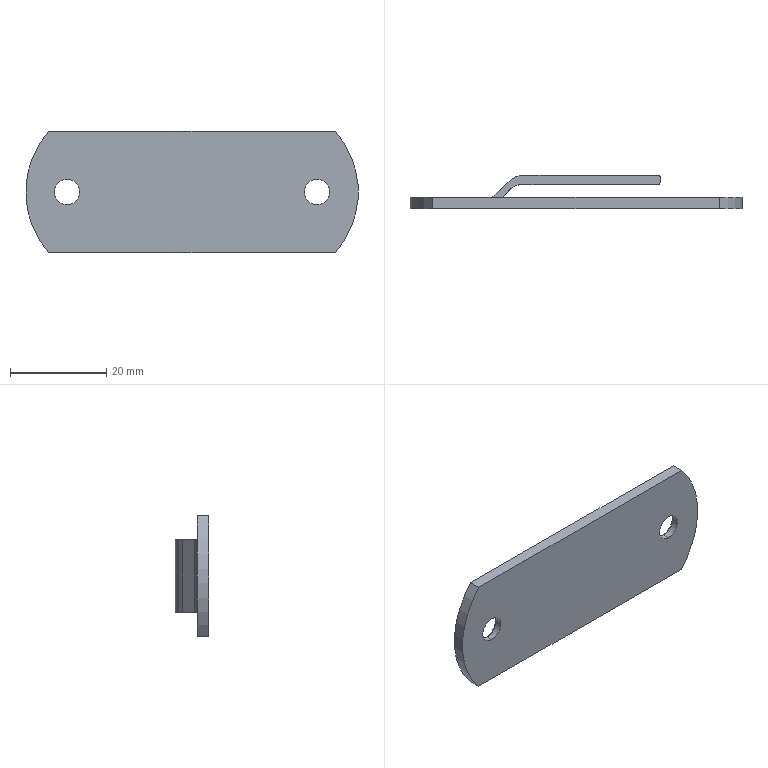Part | SolidWorks | features BaseBody 1 | 1 solid | 32 faces | box 69.2 x 7 x 25.2 mm | volume 3971 mm3 | plane 16 | cylinder 12 | cone 4 | commonest cylinder face diameters 5.3 x4 1 x2 6 x2 10 x2 37.875 x2
STEP:
#1=CARTESIAN_POINT('',(26.,-3.6,2.65));
#2=VERTEX_POINT('',#1);
#3=CARTESIAN_POINT('',(26.,-3.6,-2.65));
#4=VERTEX_POINT('',#3);
#5=CARTESIAN_POINT('',(26.,-3.6,0.));
#6=DIRECTION('',(0.,-1.,0.));
#7=DIRECTION('',(0.,0.,1.));
#8=AXIS2_PLACEMENT_3D('',#5,#6,#7);
#9=CIRCLE('',#8,2.65);
#10=EDGE_CURVE('',#2,#4,#9,.T.);
#11=ORIENTED_EDGE('',*,*,#10,.T.);
#12=CARTESIAN_POINT('',(26.,-2.2,-2.65));
#13=VERTEX_POINT('',#12);
#14=CARTESIAN_POINT('',(26.,-3.6,-2.65));
#15=DIRECTION('',(0.,1.,0.));
#16=VECTOR('',#15,1000.);
#17=LINE('',#14,#16);
#18=EDGE_CURVE('',#4,#13,#17,.T.);
#19=ORIENTED_EDGE('',*,*,#18,.T.);
#20=CARTESIAN_POINT('',(26.,-2.2,2.65));
#21=VERTEX_POINT('',#20);
#22=CARTESIAN_POINT('',(26.,-2.2,0.));
#23=DIRECTION('',(0.,-1.,0.));
#24=DIRECTION('',(0.,0.,1.));
#25=AXIS2_PLACEMENT_3D('',#22,#23,#24);
#26=CIRCLE('',#25,2.65);
#27=EDGE_CURVE('',#21,#13,#26,.T.);
#28=ORIENTED_EDGE('',*,*,#27,.F.);
#29=CARTESIAN_POINT('',(26.,-3.6,2.65));
#30=DIRECTION('',(0.,1.,0.));
#31=VECTOR('',#30,1000.);
#32=LINE('',#29,#31);
#33=EDGE_CURVE('',#2,#21,#32,.T.);
#34=ORIENTED_EDGE('',*,*,#33,.F.);
#35=EDGE_LOOP('',(#11,#19,#28,#34));
#36=FACE_OUTER_BOUND('',#35,.T.);
#37=CARTESIAN_POINT('',(26.,-3.6,0.));
#38=DIRECTION('',(0.,1.,0.));
#39=DIRECTION('',(0.,0.,1.));
#40=AXIS2_PLACEMENT_3D('',#37,#38,#39);
#41=CYLINDRICAL_SURFACE('',#40,2.65);
#42=ADVANCED_FACE('',(#36),#41,.F.);
#43=CARTESIAN_POINT('',(-26.,-3.6,2.65));
#44=VERTEX_POINT('',#43);
#45=CARTESIAN_POINT('',(-26.,-3.6,-2.65));
#46=VERTEX_POINT('',#45);
#47=CARTESIAN_POINT('',(-26.,-3.6,0.));
#48=DIRECTION('',(0.,-1.,0.));
#49=DIRECTION('',(0.,0.,1.));
#50=AXIS2_PLACEMENT_3D('',#47,#48,#49);
#51=CIRCLE('',#50,2.65);
#52=EDGE_CURVE('',#44,#46,#51,.T.);
#53=ORIENTED_EDGE('',*,*,#52,.T.);
#54=CARTESIAN_POINT('',(-26.,-2.2,-2.65));
#55=VERTEX_POINT('',#54);
#56=CARTESIAN_POINT('',(-26.,-3.6,-2.65));
#57=DIRECTION('',(0.,1.,0.));
#58=VECTOR('',#57,1000.);
#59=LINE('',#56,#58);
#60=EDGE_CURVE('',#46,#55,#59,.T.);
#61=ORIENTED_EDGE('',*,*,#60,.T.);
#62=CARTESIAN_POINT('',(-26.,-2.2,2.65));
#63=VERTEX_POINT('',#62);
#64=CARTESIAN_POINT('',(-26.,-2.2,0.));
#65=DIRECTION('',(0.,-1.,0.));
#66=DIRECTION('',(0.,0.,1.));
#67=AXIS2_PLACEMENT_3D('',#64,#65,#66);
#68=CIRCLE('',#67,2.65);
#69=EDGE_CURVE('',#63,#55,#68,.T.);
#70=ORIENTED_EDGE('',*,*,#69,.F.);
#71=CARTESIAN_POINT('',(-26.,-3.6,2.65));
#72=DIRECTION('',(0.,1.,0.));
#73=VECTOR('',#72,1000.);
#74=LINE('',#71,#73);
#75=EDGE_CURVE('',#44,#63,#74,.T.);
#76=ORIENTED_EDGE('',*,*,#75,.F.);
#77=EDGE_LOOP('',(#53,#61,#70,#76));
#78=FACE_OUTER_BOUND('',#77,.T.);
#79=CARTESIAN_POINT('',(-26.,-3.6,0.));
#80=DIRECTION('',(0.,1.,0.));
#81=DIRECTION('',(0.,0.,1.));
#82=AXIS2_PLACEMENT_3D('',#79,#80,#81);
#83=CYLINDRICAL_SURFACE('',#82,2.65);
#84=ADVANCED_FACE('',(#78),#83,.F.);
#85=ORIENTED_EDGE('',*,*,#27,.T.);
#86=CARTESIAN_POINT('',(26.,-1.2,-3.8));
#87=VERTEX_POINT('',#86);
#88=CARTESIAN_POINT('',(26.,-1.2,-3.8));
#89=DIRECTION('',(0.,0.6562,-0.7546));
#90=VECTOR('',#89,1000.);
#91=LINE('',#88,#90);
#92=EDGE_CURVE('',#13,#87,#91,.T.);
#93=ORIENTED_EDGE('',*,*,#92,.T.);
#94=CARTESIAN_POINT('',(26.,-1.2,3.8));
#95=VERTEX_POINT('',#94);
#96=CARTESIAN_POINT('',(26.,-1.2,0.));
#97=DIRECTION('',(0.,-1.,0.));
#98=DIRECTION('',(0.,0.,1.));
#99=AXIS2_PLACEMENT_3D('',#96,#97,#98);
#100=CIRCLE('',#99,3.8);
#101=EDGE_CURVE('',#95,#87,#100,.T.);
#102=ORIENTED_EDGE('',*,*,#101,.F.);
#103=CARTESIAN_POINT('',(26.,-1.2,3.8));
#104=DIRECTION('',(0.,0.6562,0.7546));
#105=VECTOR('',#104,1000.);
#106=LINE('',#103,#105);
#107=EDGE_CURVE('',#21,#95,#106,.T.);
#108=ORIENTED_EDGE('',*,*,#107,.F.);
#109=EDGE_LOOP('',(#85,#93,#102,#108));
#110=FACE_OUTER_BOUND('',#109,.T.);
#111=CARTESIAN_POINT('',(26.,-1.2,0.));
#112=DIRECTION('',(0.,1.,0.));
#113=DIRECTION('',(0.,0.,1.));
#114=AXIS2_PLACEMENT_3D('',#111,#112,#113);
#115=CONICAL_SURFACE('',#114,3.8,0.8551);
#116=ADVANCED_FACE('',(#110),#115,.F.);
#117=ORIENTED_EDGE('',*,*,#69,.T.);
#118=CARTESIAN_POINT('',(-26.,-1.2,-3.8));
#119=VERTEX_POINT('',#118);
#120=CARTESIAN_POINT('',(-26.,-1.2,-3.8));
#121=DIRECTION('',(0.,0.6562,-0.7546));
#122=VECTOR('',#121,1000.);
#123=LINE('',#120,#122);
#124=EDGE_CURVE('',#55,#119,#123,.T.);
#125=ORIENTED_EDGE('',*,*,#124,.T.);
#126=CARTESIAN_POINT('',(-26.,-1.2,3.8));
#127=VERTEX_POINT('',#126);
#128=CARTESIAN_POINT('',(-26.,-1.2,0.));
#129=DIRECTION('',(0.,-1.,0.));
#130=DIRECTION('',(0.,0.,1.));
#131=AXIS2_PLACEMENT_3D('',#128,#129,#130);
#132=CIRCLE('',#131,3.8);
#133=EDGE_CURVE('',#127,#119,#132,.T.);
#134=ORIENTED_EDGE('',*,*,#133,.F.);
#135=CARTESIAN_POINT('',(-26.,-1.2,3.8));
#136=DIRECTION('',(0.,0.6562,0.7546));
#137=VECTOR('',#136,1000.);
#138=LINE('',#135,#137);
#139=EDGE_CURVE('',#63,#127,#138,.T.);
#140=ORIENTED_EDGE('',*,*,#139,.F.);
#141=EDGE_LOOP('',(#117,#125,#134,#140));
#142=FACE_OUTER_BOUND('',#141,.T.);
#143=CARTESIAN_POINT('',(-26.,-1.2,0.));
#144=DIRECTION('',(0.,1.,0.));
#145=DIRECTION('',(0.,0.,1.));
#146=AXIS2_PLACEMENT_3D('',#143,#144,#145);
#147=CONICAL_SURFACE('',#146,3.8,0.8551);
#148=ADVANCED_FACE('',(#142),#147,.F.);
#149=CARTESIAN_POINT('',(29.8,-3.6,12.6));
#150=VERTEX_POINT('',#149);
#151=CARTESIAN_POINT('',(29.8,-3.6,-12.6));
#152=VERTEX_POINT('',#151);
#153=CARTESIAN_POINT('',(15.662,-3.6,0.));
#154=DIRECTION('',(0.,1.,0.));
#155=DIRECTION('',(0.,0.,-1.));
#156=AXIS2_PLACEMENT_3D('',#153,#154,#155);
#157=CIRCLE('',#156,18.938);
#158=EDGE_CURVE('',#150,#152,#157,.T.);
#159=ORIENTED_EDGE('',*,*,#158,.F.);
#160=CARTESIAN_POINT('',(-29.8,-3.6,12.6));
#161=VERTEX_POINT('',#160);
#162=CARTESIAN_POINT('',(-15.662,-3.6,12.6));
#163=DIRECTION('',(1.,0.,0.));
#164=VECTOR('',#163,1000.);
#165=LINE('',#162,#164);
#166=EDGE_CURVE('',#161,#150,#165,.T.);
#167=ORIENTED_EDGE('',*,*,#166,.F.);
#168=CARTESIAN_POINT('',(-29.8,-3.6,-12.6));
#169=VERTEX_POINT('',#168);
#170=CARTESIAN_POINT('',(-15.662,-3.6,0.));
#171=DIRECTION('',(0.,1.,0.));
#172=DIRECTION('',(0.,0.,-1.));
#173=AXIS2_PLACEMENT_3D('',#170,#171,#172);
#174=CIRCLE('',#173,18.938);
#175=EDGE_CURVE('',#169,#161,#174,.T.);
#176=ORIENTED_EDGE('',*,*,#175,.F.);
#177=CARTESIAN_POINT('',(-15.662,-3.6,-12.6));
#178=DIRECTION('',(-1.,0.,0.));
#179=VECTOR('',#178,1000.);
#180=LINE('',#177,#179);
#181=EDGE_CURVE('',#152,#169,#180,.T.);
#182=ORIENTED_EDGE('',*,*,#181,.F.);
#183=EDGE_LOOP('',(#159,#167,#176,#182));
#184=FACE_OUTER_BOUND('',#183,.T.);
#185=ORIENTED_EDGE('',*,*,#10,.F.);
#186=CARTESIAN_POINT('',(26.,-3.6,0.));
#187=DIRECTION('',(0.,-1.,0.));
#188=DIRECTION('',(0.,0.,1.));
#189=AXIS2_PLACEMENT_3D('',#186,#187,#188);
#190=CIRCLE('',#189,2.65);
#191=EDGE_CURVE('',#4,#2,#190,.T.);
#192=ORIENTED_EDGE('',*,*,#191,.F.);
#193=EDGE_LOOP('',(#185,#192));
#194=FACE_BOUND('',#193,.T.);
#195=ORIENTED_EDGE('',*,*,#52,.F.);
#196=CARTESIAN_POINT('',(-26.,-3.6,0.));
#197=DIRECTION('',(0.,-1.,0.));
#198=DIRECTION('',(0.,0.,1.));
#199=AXIS2_PLACEMENT_3D('',#196,#197,#198);
#200=CIRCLE('',#199,2.65);
#201=EDGE_CURVE('',#46,#44,#200,.T.);
#202=ORIENTED_EDGE('',*,*,#201,.F.);
#203=EDGE_LOOP('',(#195,#202));
#204=FACE_BOUND('',#203,.T.);
#205=CARTESIAN_POINT('',(-15.662,-3.6,0.));
#206=DIRECTION('',(0.,1.,0.));
#207=DIRECTION('',(0.,0.,1.));
#208=AXIS2_PLACEMENT_3D('',#205,#206,#207);
#209=PLANE('',#208);
#210=ADVANCED_FACE('',(#184,#194,#204),#209,.F.);
#211=ORIENTED_EDGE('',*,*,#181,.T.);
#212=CARTESIAN_POINT('',(-29.8,-1.2,-12.6));
#213=VERTEX_POINT('',#212);
#214=CARTESIAN_POINT('',(-29.8,-3.6,-12.6));
#215=DIRECTION('',(0.,1.,0.));
#216=VECTOR('',#215,1000.);
#217=LINE('',#214,#216);
#218=EDGE_CURVE('',#169,#213,#217,.T.);
#219=ORIENTED_EDGE('',*,*,#218,.T.);
#220=CARTESIAN_POINT('',(29.8,-1.2,-12.6));
#221=VERTEX_POINT('',#220);
#222=CARTESIAN_POINT('',(29.8,-1.2,-12.6));
#223=DIRECTION('',(1.,0.,0.));
#224=VECTOR('',#223,1000.);
#225=LINE('',#222,#224);
#226=EDGE_CURVE('',#213,#221,#225,.T.);
#227=ORIENTED_EDGE('',*,*,#226,.T.);
#228=CARTESIAN_POINT('',(29.8,-3.6,-12.6));
#229=DIRECTION('',(0.,-1.,0.));
#230=VECTOR('',#229,1000.);
#231=LINE('',#228,#230);
#232=EDGE_CURVE('',#221,#152,#231,.T.);
#233=ORIENTED_EDGE('',*,*,#232,.T.);
#234=EDGE_LOOP('',(#211,#219,#227,#233));
#235=FACE_OUTER_BOUND('',#234,.T.);
#236=CARTESIAN_POINT('',(29.8,-3.6,-12.6));
#237=DIRECTION('',(0.,0.,-1.));
#238=DIRECTION('',(-1.,0.,0.));
#239=AXIS2_PLACEMENT_3D('',#236,#237,#238);
#240=PLANE('',#239);
#241=ADVANCED_FACE('',(#235),#240,.T.);
#242=ORIENTED_EDGE('',*,*,#158,.T.);
#243=ORIENTED_EDGE('',*,*,#232,.F.);
#244=CARTESIAN_POINT('',(29.8,-1.2,12.6));
#245=VERTEX_POINT('',#244);
#246=CARTESIAN_POINT('',(15.662,-1.2,0.));
#247=DIRECTION('',(0.,-1.,0.));
#248=DIRECTION('',(0.,0.,-1.));
#249=AXIS2_PLACEMENT_3D('',#246,#247,#248);
#250=CIRCLE('',#249,18.938);
#251=EDGE_CURVE('',#221,#245,#250,.T.);
#252=ORIENTED_EDGE('',*,*,#251,.T.);
#253=CARTESIAN_POINT('',(29.8,-3.6,12.6));
#254=DIRECTION('',(0.,-1.,0.));
#255=VECTOR('',#254,1000.);
#256=LINE('',#253,#255);
#257=EDGE_CURVE('',#245,#150,#256,.T.);
#258=ORIENTED_EDGE('',*,*,#257,.T.);
#259=EDGE_LOOP('',(#242,#243,#252,#258));
#260=FACE_OUTER_BOUND('',#259,.T.);
#261=CARTESIAN_POINT('',(15.662,-3.6,0.));
#262=DIRECTION('',(0.,-1.,0.));
#263=DIRECTION('',(0.,0.,-1.));
#264=AXIS2_PLACEMENT_3D('',#261,#262,#263);
#265=CYLINDRICAL_SURFACE('',#264,18.938);
#266=ADVANCED_FACE('',(#260),#265,.T.);
#267=ORIENTED_EDGE('',*,*,#166,.T.);
#268=ORIENTED_EDGE('',*,*,#257,.F.);
#269=CARTESIAN_POINT('',(-29.8,-1.2,12.6));
#270=VERTEX_POINT('',#269);
#271=CARTESIAN_POINT('',(-29.8,-1.2,12.6));
#272=DIRECTION('',(-1.,0.,0.));
#273=VECTOR('',#272,1000.);
#274=LINE('',#271,#273);
#275=EDGE_CURVE('',#245,#270,#274,.T.);
#276=ORIENTED_EDGE('',*,*,#275,.T.);
#277=CARTESIAN_POINT('',(-29.8,-3.6,12.6));
#278=DIRECTION('',(0.,-1.,0.));
#279=VECTOR('',#278,1000.);
#280=LINE('',#277,#279);
#281=EDGE_CURVE('',#270,#161,#280,.T.);
#282=ORIENTED_EDGE('',*,*,#281,.T.);
#283=EDGE_LOOP('',(#267,#268,#276,#282));
#284=FACE_OUTER_BOUND('',#283,.T.);
#285=CARTESIAN_POINT('',(-29.8,-3.6,12.6));
#286=DIRECTION('',(0.,0.,1.));
#287=DIRECTION('',(1.,0.,0.));
#288=AXIS2_PLACEMENT_3D('',#285,#286,#287);
#289=PLANE('',#288);
#290=ADVANCED_FACE('',(#284),#289,.T.);
#291=ORIENTED_EDGE('',*,*,#175,.T.);
#292=ORIENTED_EDGE('',*,*,#281,.F.);
#293=CARTESIAN_POINT('',(-15.662,-1.2,0.));
#294=DIRECTION('',(0.,-1.,0.));
#295=DIRECTION('',(0.,0.,-1.));
#296=AXIS2_PLACEMENT_3D('',#293,#294,#295);
#297=CIRCLE('',#296,18.938);
#298=EDGE_CURVE('',#270,#213,#297,.T.);
#299=ORIENTED_EDGE('',*,*,#298,.T.);
#300=ORIENTED_EDGE('',*,*,#218,.F.);
#301=EDGE_LOOP('',(#291,#292,#299,#300));
#302=FACE_OUTER_BOUND('',#301,.T.);
#303=CARTESIAN_POINT('',(-15.662,-3.6,0.));
#304=DIRECTION('',(0.,-1.,0.));
#305=DIRECTION('',(0.,0.,-1.));
#306=AXIS2_PLACEMENT_3D('',#303,#304,#305);
#307=CYLINDRICAL_SURFACE('',#306,18.938);
#308=ADVANCED_FACE('',(#302),#307,.T.);
#309=ORIENTED_EDGE('',*,*,#18,.F.);
#310=ORIENTED_EDGE('',*,*,#191,.T.);
#311=ORIENTED_EDGE('',*,*,#33,.T.);
#312=CARTESIAN_POINT('',(26.,-2.2,0.));
#313=DIRECTION('',(0.,-1.,0.));
#314=DIRECTION('',(0.,0.,1.));
#315=AXIS2_PLACEMENT_3D('',#312,#313,#314);
#316=CIRCLE('',#315,2.65);
#317=EDGE_CURVE('',#13,#21,#316,.T.);
#318=ORIENTED_EDGE('',*,*,#317,.F.);
#319=EDGE_LOOP('',(#309,#310,#311,#318));
#320=FACE_OUTER_BOUND('',#319,.T.);
#321=CARTESIAN_POINT('',(26.,-3.6,0.));
#322=DIRECTION('',(0.,1.,0.));
#323=DIRECTION('',(0.,0.,1.));
#324=AXIS2_PLACEMENT_3D('',#321,#322,#323);
#325=CYLINDRICAL_SURFACE('',#324,2.65);
#326=ADVANCED_FACE('',(#320),#325,.F.);
#327=ORIENTED_EDGE('',*,*,#60,.F.);
#328=ORIENTED_EDGE('',*,*,#201,.T.);
#329=ORIENTED_EDGE('',*,*,#75,.T.);
#330=CARTESIAN_POINT('',(-26.,-2.2,0.));
#331=DIRECTION('',(0.,-1.,0.));
#332=DIRECTION('',(0.,0.,1.));
#333=AXIS2_PLACEMENT_3D('',#330,#331,#332);
#334=CIRCLE('',#333,2.65);
#335=EDGE_CURVE('',#55,#63,#334,.T.);
#336=ORIENTED_EDGE('',*,*,#335,.F.);
#337=EDGE_LOOP('',(#327,#328,#329,#336));
#338=FACE_OUTER_BOUND('',#337,.T.);
#339=CARTESIAN_POINT('',(-26.,-3.6,0.));
#340=DIRECTION('',(0.,1.,0.));
#341=DIRECTION('',(0.,0.,1.));
#342=AXIS2_PLACEMENT_3D('',#339,#340,#341);
#343=CYLINDRICAL_SURFACE('',#342,2.65);
#344=ADVANCED_FACE('',(#338),#343,.F.);
#345=ORIENTED_EDGE('',*,*,#275,.F.);
#346=ORIENTED_EDGE('',*,*,#251,.F.);
#347=ORIENTED_EDGE('',*,*,#226,.F.);
#348=ORIENTED_EDGE('',*,*,#298,.F.);
#349=EDGE_LOOP('',(#345,#346,#347,#348));
#350=FACE_OUTER_BOUND('',#349,.T.);
#351=ORIENTED_EDGE('',*,*,#101,.T.);
#352=CARTESIAN_POINT('',(26.,-1.2,0.));
#353=DIRECTION('',(0.,-1.,0.));
#354=DIRECTION('',(0.,0.,1.));
#355=AXIS2_PLACEMENT_3D('',#352,#353,#354);
#356=CIRCLE('',#355,3.8);
#357=EDGE_CURVE('',#87,#95,#356,.T.);
#358=ORIENTED_EDGE('',*,*,#357,.T.);
#359=EDGE_LOOP('',(#351,#358));
#360=FACE_BOUND('',#359,.T.);
#361=ORIENTED_EDGE('',*,*,#133,.T.);
#362=CARTESIAN_POINT('',(-26.,-1.2,0.));
#363=DIRECTION('',(0.,-1.,0.));
#364=DIRECTION('',(0.,0.,1.));
#365=AXIS2_PLACEMENT_3D('',#362,#363,#364);
#366=CIRCLE('',#365,3.8);
#367=EDGE_CURVE('',#119,#127,#366,.T.);
#368=ORIENTED_EDGE('',*,*,#367,.T.);
#369=EDGE_LOOP('',(#361,#368));
#370=FACE_BOUND('',#369,.T.);
#371=CARTESIAN_POINT('',(17.5,-1.2,-7.5));
#372=VERTEX_POINT('',#371);
#373=CARTESIAN_POINT('',(17.5,-1.2,7.5));
#374=VERTEX_POINT('',#373);
#375=CARTESIAN_POINT('',(17.5,-1.2,0.));
#376=DIRECTION('',(0.,0.,1.));
#377=VECTOR('',#376,1000.);
#378=LINE('',#375,#377);
#379=EDGE_CURVE('',#372,#374,#378,.T.);
#380=ORIENTED_EDGE('',*,*,#379,.T.);
#381=CARTESIAN_POINT('',(-15.3,-1.2,7.5));
#382=VERTEX_POINT('',#381);
#383=CARTESIAN_POINT('',(-15.662,-1.2,7.5));
#384=DIRECTION('',(-1.,0.,0.));
#385=VECTOR('',#384,1000.);
#386=LINE('',#383,#385);
#387=EDGE_CURVE('',#374,#382,#386,.T.);
#388=ORIENTED_EDGE('',*,*,#387,.T.);
#389=CARTESIAN_POINT('',(-17.666,-1.2,7.5));
#390=VERTEX_POINT('',#389);
#391=CARTESIAN_POINT('',(-15.662,-1.2,7.5));
#392=DIRECTION('',(-1.,0.,0.));
#393=VECTOR('',#392,1000.);
#394=LINE('',#391,#393);
#395=EDGE_CURVE('',#382,#390,#394,.T.);
#396=ORIENTED_EDGE('',*,*,#395,.T.);
#397=CARTESIAN_POINT('',(-17.666,-1.2,-7.5));
#398=VERTEX_POINT('',#397);
#399=CARTESIAN_POINT('',(-17.666,-1.2,0.));
#400=DIRECTION('',(0.,0.,-1.));
#401=VECTOR('',#400,1000.);
#402=LINE('',#399,#401);
#403=EDGE_CURVE('',#390,#398,#402,.T.);
#404=ORIENTED_EDGE('',*,*,#403,.T.);
#405=CARTESIAN_POINT('',(-15.3,-1.2,-7.5));
#406=VERTEX_POINT('',#405);
#407=CARTESIAN_POINT('',(-15.662,-1.2,-7.5));
#408=DIRECTION('',(1.,0.,0.));
#409=VECTOR('',#408,1000.);
#410=LINE('',#407,#409);
#411=EDGE_CURVE('',#398,#406,#410,.T.);
#412=ORIENTED_EDGE('',*,*,#411,.T.);
#413=CARTESIAN_POINT('',(-15.662,-1.2,-7.5));
#414=DIRECTION('',(1.,0.,0.));
#415=VECTOR('',#414,1000.);
#416=LINE('',#413,#415);
#417=EDGE_CURVE('',#406,#372,#416,.T.);
#418=ORIENTED_EDGE('',*,*,#417,.T.);
#419=EDGE_LOOP('',(#380,#388,#396,#404,#412,#418));
#420=FACE_BOUND('',#419,.T.);
#421=CARTESIAN_POINT('',(-15.662,-1.2,0.));
#422=DIRECTION('',(0.,1.,0.));
#423=DIRECTION('',(0.,0.,1.));
#424=AXIS2_PLACEMENT_3D('',#421,#422,#423);
#425=PLANE('',#424);
#426=ADVANCED_FACE('',(#350,#360,#370,#420),#425,.T.);
#427=ORIENTED_EDGE('',*,*,#92,.F.);
#428=ORIENTED_EDGE('',*,*,#317,.T.);
#429=ORIENTED_EDGE('',*,*,#107,.T.);
#430=ORIENTED_EDGE('',*,*,#357,.F.);
#431=EDGE_LOOP('',(#427,#428,#429,#430));
#432=FACE_OUTER_BOUND('',#431,.T.);
#433=CARTESIAN_POINT('',(26.,-1.2,0.));
#434=DIRECTION('',(0.,1.,0.));
#435=DIRECTION('',(0.,0.,1.));
#436=AXIS2_PLACEMENT_3D('',#433,#434,#435);
#437=CONICAL_SURFACE('',#436,3.8,0.8551);
#438=ADVANCED_FACE('',(#432),#437,.F.);
#439=ORIENTED_EDGE('',*,*,#124,.F.);
#440=ORIENTED_EDGE('',*,*,#335,.T.);
#441=ORIENTED_EDGE('',*,*,#139,.T.);
#442=ORIENTED_EDGE('',*,*,#367,.F.);
#443=EDGE_LOOP('',(#439,#440,#441,#442));
#444=FACE_OUTER_BOUND('',#443,.T.);
#445=CARTESIAN_POINT('',(-26.,-1.2,0.));
#446=DIRECTION('',(0.,1.,0.));
#447=DIRECTION('',(0.,0.,1.));
#448=AXIS2_PLACEMENT_3D('',#445,#446,#447);
#449=CONICAL_SURFACE('',#448,3.8,0.8551);
#450=ADVANCED_FACE('',(#444),#449,.F.);
#451=CARTESIAN_POINT('',(-16.036,-1.936,7.5));
#452=VERTEX_POINT('',#451);
#453=CARTESIAN_POINT('',(-16.036,-1.936,7.5));
#454=DIRECTION('',(0.7071,0.7071,0.));
#455=VECTOR('',#454,1000.);
#456=LINE('',#453,#455);
#457=EDGE_CURVE('',#452,#382,#456,.T.);
#458=ORIENTED_EDGE('',*,*,#457,.T.);
#459=ORIENTED_EDGE('',*,*,#387,.F.);
#460=CARTESIAN_POINT('',(17.5,-3.,7.5));
#461=VERTEX_POINT('',#460);
#462=CARTESIAN_POINT('',(17.5,0.,7.5));
#463=DIRECTION('',(0.,1.,0.));
#464=VECTOR('',#463,1000.);
#465=LINE('',#462,#464);
#466=EDGE_CURVE('',#461,#374,#465,.T.);
#467=ORIENTED_EDGE('',*,*,#466,.F.);
#468=CARTESIAN_POINT('',(-17.5,-3.,7.5));
#469=VERTEX_POINT('',#468);
#470=CARTESIAN_POINT('',(0.,-3.,7.5));
#471=DIRECTION('',(1.,0.,0.));
#472=VECTOR('',#471,1000.);
#473=LINE('',#470,#472);
#474=EDGE_CURVE('',#469,#461,#473,.T.);
#475=ORIENTED_EDGE('',*,*,#474,.F.);
#476=CARTESIAN_POINT('',(-17.5,-2.951,7.5));
#477=VERTEX_POINT('',#476);
#478=CARTESIAN_POINT('',(-17.5,3.,7.5));
#479=DIRECTION('',(0.,-1.,0.));
#480=VECTOR('',#479,1000.);
#481=LINE('',#478,#480);
#482=EDGE_CURVE('',#477,#469,#481,.T.);
#483=ORIENTED_EDGE('',*,*,#482,.F.);
#484=CARTESIAN_POINT('',(-19.571,1.6,7.5));
#485=DIRECTION('',(0.,0.,-1.));
#486=DIRECTION('',(1.,0.,0.));
#487=AXIS2_PLACEMENT_3D('',#484,#485,#486);
#488=CIRCLE('',#487,5.);
#489=EDGE_CURVE('',#452,#477,#488,.T.);
#490=ORIENTED_EDGE('',*,*,#489,.F.);
#491=EDGE_LOOP('',(#458,#459,#467,#475,#483,#490));
#492=FACE_OUTER_BOUND('',#491,.T.);
#493=CARTESIAN_POINT('',(0.,0.,7.5));
#494=DIRECTION('',(0.,0.,1.));
#495=DIRECTION('',(1.,0.,0.));
#496=AXIS2_PLACEMENT_3D('',#493,#494,#495);
#497=PLANE('',#496);
#498=ADVANCED_FACE('',(#492),#497,.F.);
#499=ORIENTED_EDGE('',*,*,#466,.T.);
#500=ORIENTED_EDGE('',*,*,#379,.F.);
#501=CARTESIAN_POINT('',(17.5,-3.,-7.5));
#502=VERTEX_POINT('',#501);
#503=CARTESIAN_POINT('',(17.5,-3.,-7.5));
#504=DIRECTION('',(0.,-1.,0.));
#505=VECTOR('',#504,1000.);
#506=LINE('',#503,#505);
#507=EDGE_CURVE('',#372,#502,#506,.T.);
#508=ORIENTED_EDGE('',*,*,#507,.T.);
#509=CARTESIAN_POINT('',(17.5,-3.,7.5));
#510=DIRECTION('',(0.,0.,1.));
#511=VECTOR('',#510,1000.);
#512=LINE('',#509,#511);
#513=EDGE_CURVE('',#502,#461,#512,.T.);
#514=ORIENTED_EDGE('',*,*,#513,.T.);
#515=EDGE_LOOP('',(#499,#500,#508,#514));
#516=FACE_OUTER_BOUND('',#515,.T.);
#517=CARTESIAN_POINT('',(17.5,-3.,7.5));
#518=DIRECTION('',(-1.,0.,0.));
#519=DIRECTION('',(0.,0.,1.));
#520=AXIS2_PLACEMENT_3D('',#517,#518,#519);
#521=PLANE('',#520);
#522=ADVANCED_FACE('',(#516),#521,.T.);
#523=ORIENTED_EDGE('',*,*,#507,.F.);
#524=ORIENTED_EDGE('',*,*,#417,.F.);
#525=CARTESIAN_POINT('',(-16.036,-1.936,-7.5));
#526=VERTEX_POINT('',#525);
#527=CARTESIAN_POINT('',(-16.036,-1.936,-7.5));
#528=DIRECTION('',(-0.7071,-0.7071,0.));
#529=VECTOR('',#528,1000.);
#530=LINE('',#527,#529);
#531=EDGE_CURVE('',#406,#526,#530,.T.);
#532=ORIENTED_EDGE('',*,*,#531,.T.);
#533=CARTESIAN_POINT('',(-17.5,-2.951,-7.5));
#534=VERTEX_POINT('',#533);
#535=CARTESIAN_POINT('',(-19.571,1.6,-7.5));
#536=DIRECTION('',(0.,0.,-1.));
#537=DIRECTION('',(1.,0.,0.));
#538=AXIS2_PLACEMENT_3D('',#535,#536,#537);
#539=CIRCLE('',#538,5.);
#540=EDGE_CURVE('',#526,#534,#539,.T.);
#541=ORIENTED_EDGE('',*,*,#540,.T.);
#542=CARTESIAN_POINT('',(-17.5,-3.,-7.5));
#543=VERTEX_POINT('',#542);
#544=CARTESIAN_POINT('',(-17.5,3.,-7.5));
#545=DIRECTION('',(0.,1.,0.));
#546=VECTOR('',#545,1000.);
#547=LINE('',#544,#546);
#548=EDGE_CURVE('',#543,#534,#547,.T.);
#549=ORIENTED_EDGE('',*,*,#548,.F.);
#550=CARTESIAN_POINT('',(0.,-3.,-7.5));
#551=DIRECTION('',(1.,0.,0.));
#552=VECTOR('',#551,1000.);
#553=LINE('',#550,#552);
#554=EDGE_CURVE('',#543,#502,#553,.T.);
#555=ORIENTED_EDGE('',*,*,#554,.T.);
#556=EDGE_LOOP('',(#523,#524,#532,#541,#549,#555));
#557=FACE_OUTER_BOUND('',#556,.T.);
#558=CARTESIAN_POINT('',(0.,0.,-7.5));
#559=DIRECTION('',(0.,0.,1.));
#560=DIRECTION('',(1.,0.,0.));
#561=AXIS2_PLACEMENT_3D('',#558,#559,#560);
#562=PLANE('',#561);
#563=ADVANCED_FACE('',(#557),#562,.T.);
#564=CARTESIAN_POINT('',(-16.621,-0.5213,-7.5));
#565=VERTEX_POINT('',#564);
#566=CARTESIAN_POINT('',(-18.743,1.6,-7.5));
#567=DIRECTION('',(0.,0.,-1.));
#568=DIRECTION('',(1.,0.,0.));
#569=AXIS2_PLACEMENT_3D('',#566,#567,#568);
#570=CIRCLE('',#569,3.);
#571=EDGE_CURVE('',#565,#398,#570,.T.);
#572=ORIENTED_EDGE('',*,*,#571,.F.);
#573=CARTESIAN_POINT('',(-14.164,1.936,-7.5));
#574=VERTEX_POINT('',#573);
#575=CARTESIAN_POINT('',(-14.164,1.936,-7.5));
#576=DIRECTION('',(-0.7071,-0.7071,0.));
#577=VECTOR('',#576,1000.);
#578=LINE('',#575,#577);
#579=EDGE_CURVE('',#574,#565,#578,.T.);
#580=ORIENTED_EDGE('',*,*,#579,.F.);
#581=CARTESIAN_POINT('',(-10.629,3.4,-7.5));
#582=VERTEX_POINT('',#581);
#583=CARTESIAN_POINT('',(-10.629,-1.6,-7.5));
#584=DIRECTION('',(0.,0.,1.));
#585=DIRECTION('',(1.,0.,0.));
#586=AXIS2_PLACEMENT_3D('',#583,#584,#585);
#587=CIRCLE('',#586,5.);
#588=EDGE_CURVE('',#582,#574,#587,.T.);
#589=ORIENTED_EDGE('',*,*,#588,.F.);
#590=CARTESIAN_POINT('',(17.,3.4,-7.5));
#591=VERTEX_POINT('',#590);
#592=CARTESIAN_POINT('',(-19.571,3.4,-7.5));
#593=DIRECTION('',(-1.,0.,0.));
#594=VECTOR('',#593,1000.);
#595=LINE('',#592,#594);
#596=EDGE_CURVE('',#591,#582,#595,.T.);
#597=ORIENTED_EDGE('',*,*,#596,.F.);
#598=CARTESIAN_POINT('',(17.5,2.9,-7.5));
#599=VERTEX_POINT('',#598);
#600=CARTESIAN_POINT('',(17.,2.9,-7.5));
#601=DIRECTION('',(0.,0.,1.));
#602=DIRECTION('',(1.,0.,0.));
#603=AXIS2_PLACEMENT_3D('',#600,#601,#602);
#604=CIRCLE('',#603,0.5);
#605=EDGE_CURVE('',#599,#591,#604,.T.);
#606=ORIENTED_EDGE('',*,*,#605,.F.);
#607=CARTESIAN_POINT('',(17.5,1.9,-7.5));
#608=VERTEX_POINT('',#607);
#609=CARTESIAN_POINT('',(17.5,1.9,-7.5));
#610=DIRECTION('',(0.,-1.,0.));
#611=VECTOR('',#610,1000.);
#612=LINE('',#609,#611);
#613=EDGE_CURVE('',#599,#608,#612,.T.);
#614=ORIENTED_EDGE('',*,*,#613,.T.);
#615=CARTESIAN_POINT('',(17.,1.4,-7.5));
#616=VERTEX_POINT('',#615);
#617=CARTESIAN_POINT('',(17.,1.9,-7.5));
#618=DIRECTION('',(0.,0.,1.));
#619=DIRECTION('',(1.,0.,0.));
#620=AXIS2_PLACEMENT_3D('',#617,#618,#619);
#621=CIRCLE('',#620,0.5);
#622=EDGE_CURVE('',#616,#608,#621,.T.);
#623=ORIENTED_EDGE('',*,*,#622,.F.);
#624=CARTESIAN_POINT('',(-11.457,1.4,-7.5));
#625=VERTEX_POINT('',#624);
#626=CARTESIAN_POINT('',(-19.571,1.4,-7.5));
#627=DIRECTION('',(1.,0.,0.));
#628=VECTOR('',#627,1000.);
#629=LINE('',#626,#628);
#630=EDGE_CURVE('',#625,#616,#629,.T.);
#631=ORIENTED_EDGE('',*,*,#630,.F.);
#632=CARTESIAN_POINT('',(-13.579,0.5213,-7.5));
#633=VERTEX_POINT('',#632);
#634=CARTESIAN_POINT('',(-11.457,-1.6,-7.5));
#635=DIRECTION('',(0.,0.,-1.));
#636=DIRECTION('',(1.,0.,0.));
#637=AXIS2_PLACEMENT_3D('',#634,#635,#636);
#638=CIRCLE('',#637,3.);
#639=EDGE_CURVE('',#633,#625,#638,.T.);
#640=ORIENTED_EDGE('',*,*,#639,.F.);
#641=CARTESIAN_POINT('',(-15.3,-1.2,-7.5));
#642=DIRECTION('',(0.7071,0.7071,0.));
#643=VECTOR('',#642,1000.);
#644=LINE('',#641,#643);
#645=EDGE_CURVE('',#406,#633,#644,.T.);
#646=ORIENTED_EDGE('',*,*,#645,.F.);
#647=ORIENTED_EDGE('',*,*,#411,.F.);
#648=EDGE_LOOP('',(#572,#580,#589,#597,#606,#614,#623,#631,#640,#646,#647));
#649=FACE_OUTER_BOUND('',#648,.T.);
#650=CARTESIAN_POINT('',(-19.571,1.6,-7.5));
#651=DIRECTION('',(0.,0.,1.));
#652=DIRECTION('',(1.,0.,0.));
#653=AXIS2_PLACEMENT_3D('',#650,#651,#652);
#654=PLANE('',#653);
#655=ADVANCED_FACE('',(#649),#654,.F.);
#656=ORIENTED_EDGE('',*,*,#403,.F.);
#657=CARTESIAN_POINT('',(-16.621,-0.5213,7.5));
#658=VERTEX_POINT('',#657);
#659=CARTESIAN_POINT('',(-18.743,1.6,7.5));
#660=DIRECTION('',(0.,0.,-1.));
#661=DIRECTION('',(1.,0.,0.));
#662=AXIS2_PLACEMENT_3D('',#659,#660,#661);
#663=CIRCLE('',#662,3.);
#664=EDGE_CURVE('',#658,#390,#663,.T.);
#665=ORIENTED_EDGE('',*,*,#664,.F.);
#666=CARTESIAN_POINT('',(-16.621,-0.5213,7.5));
#667=DIRECTION('',(0.,0.,1.));
#668=VECTOR('',#667,1000.);
#669=LINE('',#666,#668);
#670=EDGE_CURVE('',#565,#658,#669,.T.);
#671=ORIENTED_EDGE('',*,*,#670,.F.);
#672=ORIENTED_EDGE('',*,*,#571,.T.);
#673=EDGE_LOOP('',(#656,#665,#671,#672));
#674=FACE_OUTER_BOUND('',#673,.T.);
#675=CARTESIAN_POINT('',(-18.743,1.6,7.5));
#676=DIRECTION('',(0.,0.,1.));
#677=DIRECTION('',(1.,0.,0.));
#678=AXIS2_PLACEMENT_3D('',#675,#676,#677);
#679=CYLINDRICAL_SURFACE('',#678,3.);
#680=ADVANCED_FACE('',(#674),#679,.F.);
#681=CARTESIAN_POINT('',(-10.629,3.4,7.5));
#682=VERTEX_POINT('',#681);
#683=CARTESIAN_POINT('',(-14.164,1.936,7.5));
#684=VERTEX_POINT('',#683);
#685=CARTESIAN_POINT('',(-10.629,-1.6,7.5));
#686=DIRECTION('',(0.,0.,1.));
#687=DIRECTION('',(1.,0.,0.));
#688=AXIS2_PLACEMENT_3D('',#685,#686,#687);
#689=CIRCLE('',#688,5.);
#690=EDGE_CURVE('',#682,#684,#689,.T.);
#691=ORIENTED_EDGE('',*,*,#690,.T.);
#692=CARTESIAN_POINT('',(-14.164,1.936,7.5));
#693=DIRECTION('',(-0.7071,-0.7071,0.));
#694=VECTOR('',#693,1000.);
#695=LINE('',#692,#694);
#696=EDGE_CURVE('',#684,#658,#695,.T.);
#697=ORIENTED_EDGE('',*,*,#696,.T.);
#698=ORIENTED_EDGE('',*,*,#664,.T.);
#699=ORIENTED_EDGE('',*,*,#395,.F.);
#700=CARTESIAN_POINT('',(-13.579,0.5213,7.5));
#701=VERTEX_POINT('',#700);
#702=CARTESIAN_POINT('',(-15.3,-1.2,7.5));
#703=DIRECTION('',(0.7071,0.7071,0.));
#704=VECTOR('',#703,1000.);
#705=LINE('',#702,#704);
#706=EDGE_CURVE('',#382,#701,#705,.T.);
#707=ORIENTED_EDGE('',*,*,#706,.T.);
#708=CARTESIAN_POINT('',(-11.457,1.4,7.5));
#709=VERTEX_POINT('',#708);
#710=CARTESIAN_POINT('',(-11.457,-1.6,7.5));
#711=DIRECTION('',(0.,0.,-1.));
#712=DIRECTION('',(1.,0.,0.));
#713=AXIS2_PLACEMENT_3D('',#710,#711,#712);
#714=CIRCLE('',#713,3.);
#715=EDGE_CURVE('',#701,#709,#714,.T.);
#716=ORIENTED_EDGE('',*,*,#715,.T.);
#717=CARTESIAN_POINT('',(17.,1.4,7.5));
#718=VERTEX_POINT('',#717);
#719=CARTESIAN_POINT('',(-19.571,1.4,7.5));
#720=DIRECTION('',(1.,0.,0.));
#721=VECTOR('',#720,1000.);
#722=LINE('',#719,#721);
#723=EDGE_CURVE('',#709,#718,#722,.T.);
#724=ORIENTED_EDGE('',*,*,#723,.T.);
#725=CARTESIAN_POINT('',(17.5,1.9,7.5));
#726=VERTEX_POINT('',#725);
#727=CARTESIAN_POINT('',(17.,1.9,7.5));
#728=DIRECTION('',(0.,0.,-1.));
#729=DIRECTION('',(1.,0.,0.));
#730=AXIS2_PLACEMENT_3D('',#727,#728,#729);
#731=CIRCLE('',#730,0.5);
#732=EDGE_CURVE('',#726,#718,#731,.T.);
#733=ORIENTED_EDGE('',*,*,#732,.F.);
#734=CARTESIAN_POINT('',(17.5,2.9,7.5));
#735=VERTEX_POINT('',#734);
#736=CARTESIAN_POINT('',(17.5,1.9,7.5));
#737=DIRECTION('',(0.,1.,0.));
#738=VECTOR('',#737,1000.);
#739=LINE('',#736,#738);
#740=EDGE_CURVE('',#726,#735,#739,.T.);
#741=ORIENTED_EDGE('',*,*,#740,.T.);
#742=CARTESIAN_POINT('',(17.,3.4,7.5));
#743=VERTEX_POINT('',#742);
#744=CARTESIAN_POINT('',(17.,2.9,7.5));
#745=DIRECTION('',(0.,0.,-1.));
#746=DIRECTION('',(1.,0.,0.));
#747=AXIS2_PLACEMENT_3D('',#744,#745,#746);
#748=CIRCLE('',#747,0.5);
#749=EDGE_CURVE('',#743,#735,#748,.T.);
#750=ORIENTED_EDGE('',*,*,#749,.F.);
#751=CARTESIAN_POINT('',(-19.571,3.4,7.5));
#752=DIRECTION('',(-1.,0.,0.));
#753=VECTOR('',#752,1000.);
#754=LINE('',#751,#753);
#755=EDGE_CURVE('',#743,#682,#754,.T.);
#756=ORIENTED_EDGE('',*,*,#755,.T.);
#757=EDGE_LOOP('',(#691,#697,#698,#699,#707,#716,#724,#733,#741,#750,#756));
#758=FACE_OUTER_BOUND('',#757,.T.);
#759=CARTESIAN_POINT('',(-19.571,1.6,7.5));
#760=DIRECTION('',(0.,0.,1.));
#761=DIRECTION('',(1.,0.,0.));
#762=AXIS2_PLACEMENT_3D('',#759,#760,#761);
#763=PLANE('',#762);
#764=ADVANCED_FACE('',(#758),#763,.T.);
#765=CARTESIAN_POINT('',(-16.036,-1.936,7.5));
#766=DIRECTION('',(0.,0.,1.));
#767=VECTOR('',#766,1000.);
#768=LINE('',#765,#767);
#769=EDGE_CURVE('',#526,#452,#768,.T.);
#770=ORIENTED_EDGE('',*,*,#769,.T.);
#771=ORIENTED_EDGE('',*,*,#489,.T.);
#772=CARTESIAN_POINT('',(-17.5,-2.951,7.5));
#773=DIRECTION('',(0.,0.,-1.));
#774=VECTOR('',#773,1000.);
#775=LINE('',#772,#774);
#776=EDGE_CURVE('',#477,#534,#775,.T.);
#777=ORIENTED_EDGE('',*,*,#776,.T.);
#778=ORIENTED_EDGE('',*,*,#540,.F.);
#779=EDGE_LOOP('',(#770,#771,#777,#778));
#780=FACE_OUTER_BOUND('',#779,.T.);
#781=CARTESIAN_POINT('',(-19.571,1.6,7.5));
#782=DIRECTION('',(0.,0.,1.));
#783=DIRECTION('',(1.,0.,0.));
#784=AXIS2_PLACEMENT_3D('',#781,#782,#783);
#785=CYLINDRICAL_SURFACE('',#784,5.);
#786=ADVANCED_FACE('',(#780),#785,.T.);
#787=ORIENTED_EDGE('',*,*,#474,.T.);
#788=ORIENTED_EDGE('',*,*,#513,.F.);
#789=ORIENTED_EDGE('',*,*,#554,.F.);
#790=CARTESIAN_POINT('',(-17.5,-3.,7.5));
#791=DIRECTION('',(0.,0.,1.));
#792=VECTOR('',#791,1000.);
#793=LINE('',#790,#792);
#794=EDGE_CURVE('',#543,#469,#793,.T.);
#795=ORIENTED_EDGE('',*,*,#794,.T.);
#796=EDGE_LOOP('',(#787,#788,#789,#795));
#797=FACE_OUTER_BOUND('',#796,.T.);
#798=CARTESIAN_POINT('',(-17.5,-3.,7.5));
#799=DIRECTION('',(0.,1.,0.));
#800=DIRECTION('',(0.,0.,1.));
#801=AXIS2_PLACEMENT_3D('',#798,#799,#800);
#802=PLANE('',#801);
#803=ADVANCED_FACE('',(#797),#802,.T.);
#804=ORIENTED_EDGE('',*,*,#670,.T.);
#805=ORIENTED_EDGE('',*,*,#696,.F.);
#806=CARTESIAN_POINT('',(-14.164,1.936,7.5));
#807=DIRECTION('',(0.,0.,1.));
#808=VECTOR('',#807,1000.);
#809=LINE('',#806,#808);
#810=EDGE_CURVE('',#574,#684,#809,.T.);
#811=ORIENTED_EDGE('',*,*,#810,.F.);
#812=ORIENTED_EDGE('',*,*,#579,.T.);
#813=EDGE_LOOP('',(#804,#805,#811,#812));
#814=FACE_OUTER_BOUND('',#813,.T.);
#815=CARTESIAN_POINT('',(-14.164,1.936,7.5));
#816=DIRECTION('',(0.7071,-0.7071,0.));
#817=DIRECTION('',(0.7071,0.7071,0.));
#818=AXIS2_PLACEMENT_3D('',#815,#816,#817);
#819=PLANE('',#818);
#820=ADVANCED_FACE('',(#814),#819,.F.);
#821=ORIENTED_EDGE('',*,*,#690,.F.);
#822=CARTESIAN_POINT('',(-10.629,3.4,7.5));
#823=DIRECTION('',(0.,0.,-1.));
#824=VECTOR('',#823,1000.);
#825=LINE('',#822,#824);
#826=EDGE_CURVE('',#682,#582,#825,.T.);
#827=ORIENTED_EDGE('',*,*,#826,.T.);
#828=ORIENTED_EDGE('',*,*,#588,.T.);
#829=ORIENTED_EDGE('',*,*,#810,.T.);
#830=EDGE_LOOP('',(#821,#827,#828,#829));
#831=FACE_OUTER_BOUND('',#830,.T.);
#832=CARTESIAN_POINT('',(-10.629,-1.6,7.5));
#833=DIRECTION('',(0.,0.,1.));
#834=DIRECTION('',(1.,0.,0.));
#835=AXIS2_PLACEMENT_3D('',#832,#833,#834);
#836=CYLINDRICAL_SURFACE('',#835,5.);
#837=ADVANCED_FACE('',(#831),#836,.T.);
#838=ORIENTED_EDGE('',*,*,#826,.F.);
#839=ORIENTED_EDGE('',*,*,#755,.F.);
#840=CARTESIAN_POINT('',(17.,3.4,7.5));
#841=DIRECTION('',(0.,0.,1.));
#842=VECTOR('',#841,1000.);
#843=LINE('',#840,#842);
#844=EDGE_CURVE('',#591,#743,#843,.T.);
#845=ORIENTED_EDGE('',*,*,#844,.F.);
#846=ORIENTED_EDGE('',*,*,#596,.T.);
#847=EDGE_LOOP('',(#838,#839,#845,#846));
#848=FACE_OUTER_BOUND('',#847,.T.);
#849=CARTESIAN_POINT('',(17.,3.4,7.5));
#850=DIRECTION('',(0.,-1.,0.));
#851=DIRECTION('',(0.,0.,-1.));
#852=AXIS2_PLACEMENT_3D('',#849,#850,#851);
#853=PLANE('',#852);
#854=ADVANCED_FACE('',(#848),#853,.F.);
#855=CARTESIAN_POINT('',(17.,1.4,7.5));
#856=DIRECTION('',(0.,0.,-1.));
#857=VECTOR('',#856,1000.);
#858=LINE('',#855,#857);
#859=EDGE_CURVE('',#718,#616,#858,.T.);
#860=ORIENTED_EDGE('',*,*,#859,.F.);
#861=ORIENTED_EDGE('',*,*,#723,.F.);
#862=CARTESIAN_POINT('',(-11.457,1.4,7.5));
#863=DIRECTION('',(0.,0.,1.));
#864=VECTOR('',#863,1000.);
#865=LINE('',#862,#864);
#866=EDGE_CURVE('',#625,#709,#865,.T.);
#867=ORIENTED_EDGE('',*,*,#866,.F.);
#868=ORIENTED_EDGE('',*,*,#630,.T.);
#869=EDGE_LOOP('',(#860,#861,#867,#868));
#870=FACE_OUTER_BOUND('',#869,.T.);
#871=CARTESIAN_POINT('',(-11.457,1.4,7.5));
#872=DIRECTION('',(0.,1.,0.));
#873=DIRECTION('',(0.,0.,1.));
#874=AXIS2_PLACEMENT_3D('',#871,#872,#873);
#875=PLANE('',#874);
#876=ADVANCED_FACE('',(#870),#875,.F.);
#877=ORIENTED_EDGE('',*,*,#866,.T.);
#878=ORIENTED_EDGE('',*,*,#715,.F.);
#879=CARTESIAN_POINT('',(-13.579,0.5213,7.5));
#880=DIRECTION('',(0.,0.,1.));
#881=VECTOR('',#880,1000.);
#882=LINE('',#879,#881);
#883=EDGE_CURVE('',#633,#701,#882,.T.);
#884=ORIENTED_EDGE('',*,*,#883,.F.);
#885=ORIENTED_EDGE('',*,*,#639,.T.);
#886=EDGE_LOOP('',(#877,#878,#884,#885));
#887=FACE_OUTER_BOUND('',#886,.T.);
#888=CARTESIAN_POINT('',(-11.457,-1.6,7.5));
#889=DIRECTION('',(0.,0.,1.));
#890=DIRECTION('',(1.,0.,0.));
#891=AXIS2_PLACEMENT_3D('',#888,#889,#890);
#892=CYLINDRICAL_SURFACE('',#891,3.);
#893=ADVANCED_FACE('',(#887),#892,.F.);
#894=ORIENTED_EDGE('',*,*,#645,.T.);
#895=ORIENTED_EDGE('',*,*,#883,.T.);
#896=ORIENTED_EDGE('',*,*,#706,.F.);
#897=ORIENTED_EDGE('',*,*,#457,.F.);
#898=ORIENTED_EDGE('',*,*,#769,.F.);
#899=ORIENTED_EDGE('',*,*,#531,.F.);
#900=EDGE_LOOP('',(#894,#895,#896,#897,#898,#899));
#901=FACE_OUTER_BOUND('',#900,.T.);
#902=CARTESIAN_POINT('',(-16.036,-1.936,7.5));
#903=DIRECTION('',(-0.7071,0.7071,0.));
#904=DIRECTION('',(-0.7071,-0.7071,0.));
#905=AXIS2_PLACEMENT_3D('',#902,#903,#904);
#906=PLANE('',#905);
#907=ADVANCED_FACE('',(#901),#906,.F.);
#908=ORIENTED_EDGE('',*,*,#482,.T.);
#909=ORIENTED_EDGE('',*,*,#794,.F.);
#910=ORIENTED_EDGE('',*,*,#548,.T.);
#911=ORIENTED_EDGE('',*,*,#776,.F.);
#912=EDGE_LOOP('',(#908,#909,#910,#911));
#913=FACE_OUTER_BOUND('',#912,.T.);
#914=CARTESIAN_POINT('',(-17.5,3.,7.5));
#915=DIRECTION('',(1.,0.,0.));
#916=DIRECTION('',(0.,0.,-1.));
#917=AXIS2_PLACEMENT_3D('',#914,#915,#916);
#918=PLANE('',#917);
#919=ADVANCED_FACE('',(#913),#918,.T.);
#920=ORIENTED_EDGE('',*,*,#749,.T.);
#921=CARTESIAN_POINT('',(17.5,2.9,7.5));
#922=DIRECTION('',(0.,0.,-1.));
#923=VECTOR('',#922,1000.);
#924=LINE('',#921,#923);
#925=EDGE_CURVE('',#735,#599,#924,.T.);
#926=ORIENTED_EDGE('',*,*,#925,.T.);
#927=ORIENTED_EDGE('',*,*,#605,.T.);
#928=ORIENTED_EDGE('',*,*,#844,.T.);
#929=EDGE_LOOP('',(#920,#926,#927,#928));
#930=FACE_OUTER_BOUND('',#929,.T.);
#931=CARTESIAN_POINT('',(17.,2.9,7.5));
#932=DIRECTION('',(0.,0.,1.));
#933=DIRECTION('',(1.,0.,0.));
#934=AXIS2_PLACEMENT_3D('',#931,#932,#933);
#935=CYLINDRICAL_SURFACE('',#934,0.5);
#936=ADVANCED_FACE('',(#930),#935,.T.);
#937=ORIENTED_EDGE('',*,*,#732,.T.);
#938=ORIENTED_EDGE('',*,*,#859,.T.);
#939=ORIENTED_EDGE('',*,*,#622,.T.);
#940=CARTESIAN_POINT('',(17.5,1.9,7.5));
#941=DIRECTION('',(0.,0.,1.));
#942=VECTOR('',#941,1000.);
#943=LINE('',#940,#942);
#944=EDGE_CURVE('',#608,#726,#943,.T.);
#945=ORIENTED_EDGE('',*,*,#944,.T.);
#946=EDGE_LOOP('',(#937,#938,#939,#945));
#947=FACE_OUTER_BOUND('',#946,.T.);
#948=CARTESIAN_POINT('',(17.,1.9,7.5));
#949=DIRECTION('',(0.,0.,1.));
#950=DIRECTION('',(1.,0.,0.));
#951=AXIS2_PLACEMENT_3D('',#948,#949,#950);
#952=CYLINDRICAL_SURFACE('',#951,0.5);
#953=ADVANCED_FACE('',(#947),#952,.T.);
#954=ORIENTED_EDGE('',*,*,#925,.F.);
#955=ORIENTED_EDGE('',*,*,#740,.F.);
#956=ORIENTED_EDGE('',*,*,#944,.F.);
#957=ORIENTED_EDGE('',*,*,#613,.F.);
#958=EDGE_LOOP('',(#954,#955,#956,#957));
#959=FACE_OUTER_BOUND('',#958,.T.);
#960=CARTESIAN_POINT('',(17.5,1.9,7.5));
#961=DIRECTION('',(-1.,0.,0.));
#962=DIRECTION('',(0.,0.,1.));
#963=AXIS2_PLACEMENT_3D('',#960,#961,#962);
#964=PLANE('',#963);
#965=ADVANCED_FACE('',(#959),#964,.F.);
#966=CLOSED_SHELL('',(#42,#84,#116,#148,#210,#241,#266,#290,#308,#326,#344,#426,#438,#450,#498,#522,#563,#655,#680,#764,#786,#803,#820,#837,#854,#876,#893,#907,#919,#936,#953,#965));
#967=MANIFOLD_SOLID_BREP('',#966);
#968=CARTESIAN_POINT('',(0.,0.,0.));
#969=DIRECTION('',(0.,0.,1.));
#970=DIRECTION('',(1.,0.,0.));
#971=AXIS2_PLACEMENT_3D('',#968,#969,#970);
#972=(LENGTH_UNIT()NAMED_UNIT(*)SI_UNIT(.MILLI.,.METRE.));
#973=UNCERTAINTY_MEASURE_WITH_UNIT(LENGTH_MEASURE(0.00001),#972,'','');
#974=(NAMED_UNIT(*)PLANE_ANGLE_UNIT()SI_UNIT($,.RADIAN.));
#975=(NAMED_UNIT(*)SI_UNIT($,.STERADIAN.)SOLID_ANGLE_UNIT());
#976=(GEOMETRIC_REPRESENTATION_CONTEXT(3)GLOBAL_UNCERTAINTY_ASSIGNED_CONTEXT((#973))GLOBAL_UNIT_ASSIGNED_CONTEXT((#972,#974,#975))REPRESENTATION_CONTEXT('',''));
#977=ADVANCED_BREP_SHAPE_REPRESENTATION('',(#967,#971),#976);